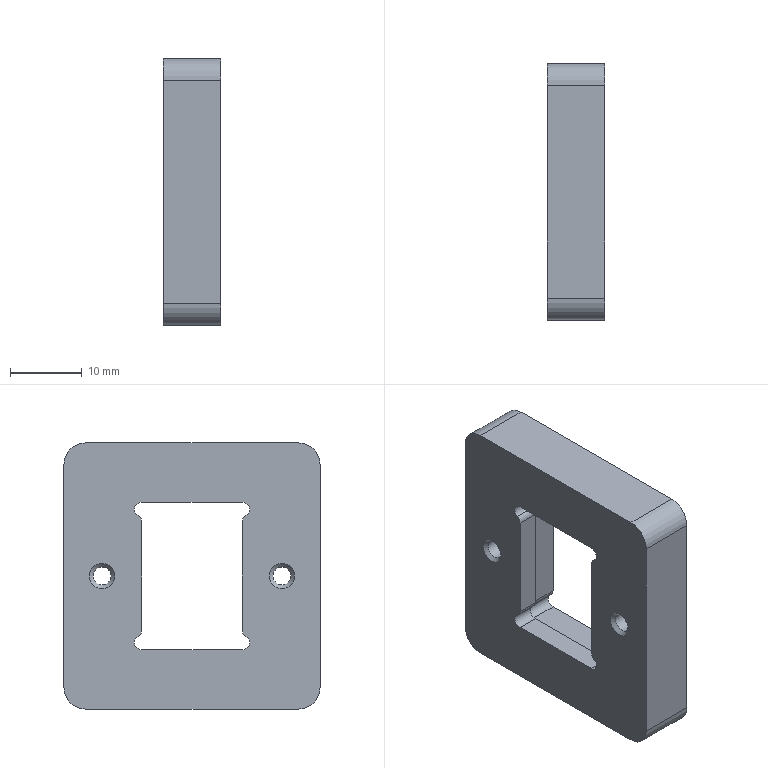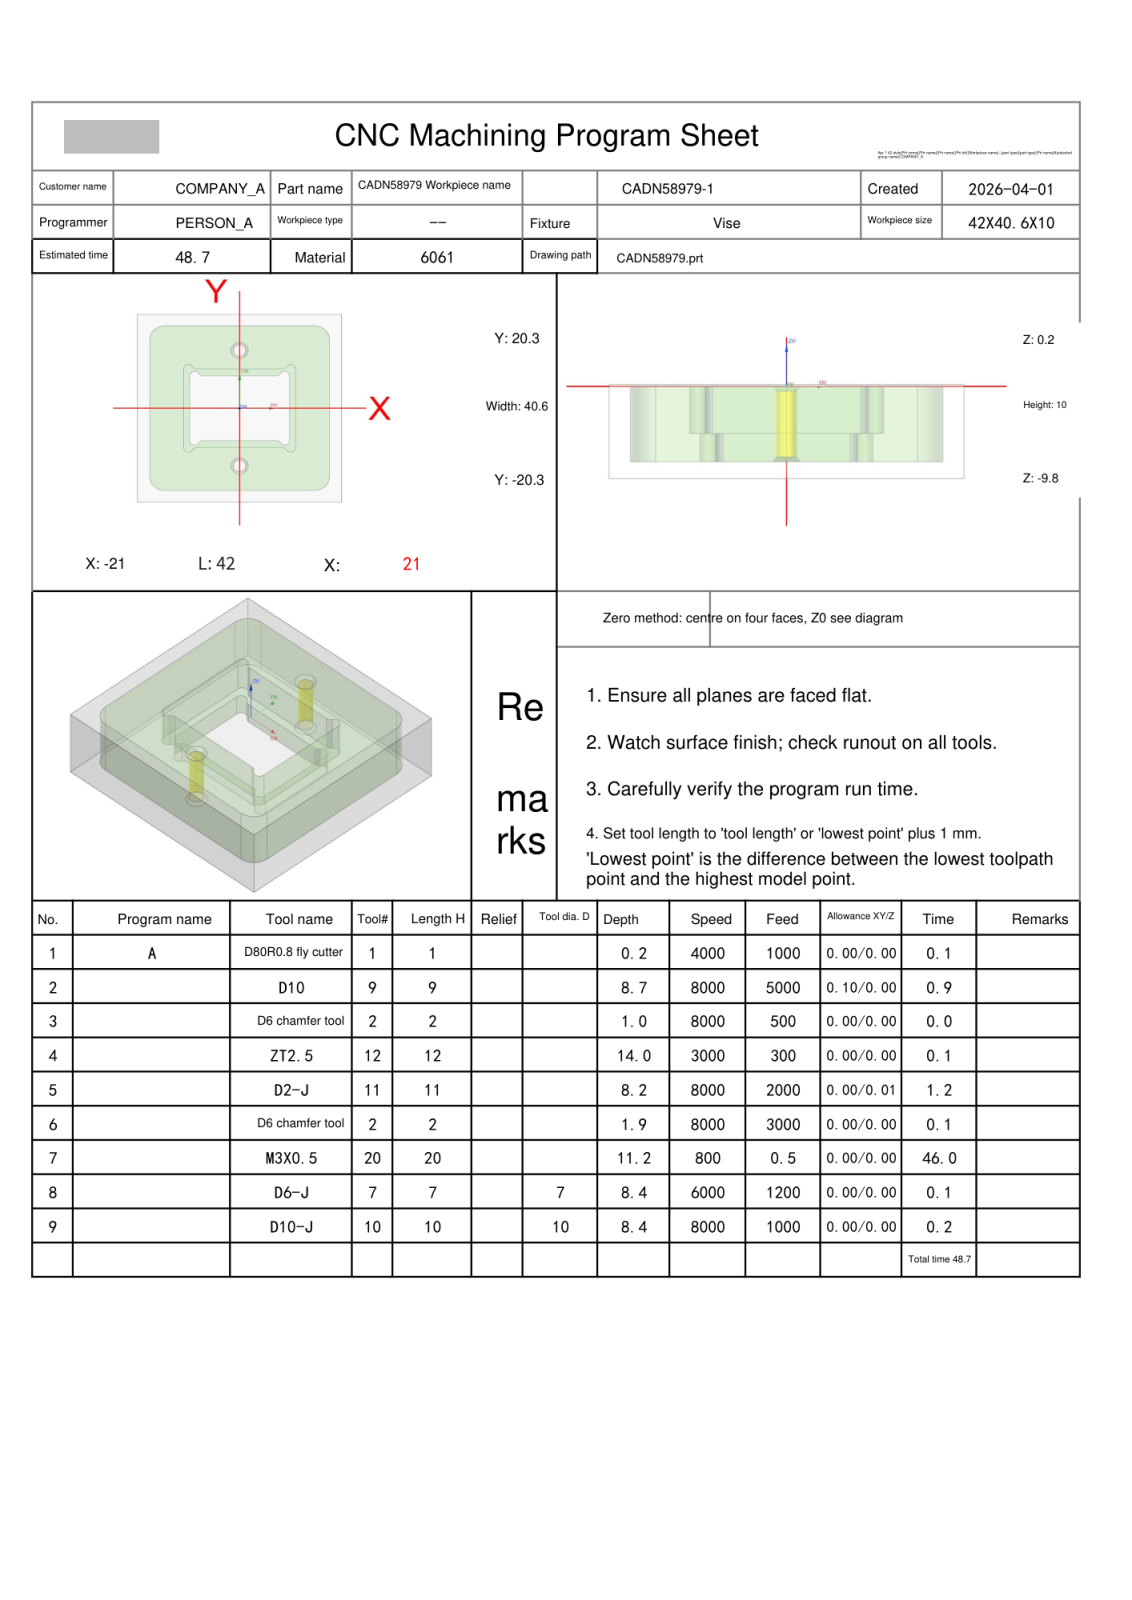NC program | NX | posted by the shop | part box 8 x 35.6 x 37 mm
Lines 3801 to 3954 of 3954:
N6 T02 M06
(D6 chamfer tool  D=6. R=0. H=02 ce=0.00 di=0.00)
G00 G90 G54 X.25 Y-19.928 M03 S8000
G43 H02 Z20.
M08
Z2.099
G01 Z-1.5 F3000.
G03 X.33 Y-19.628 I-.52 J.3
X.03 Y-19.108 I-.6 J0.0
G01 X0.0 Y-19.1
X-15.5
G02 X-19.8 Y-14.8 I0.0 J4.3
G01 Y14.8
G02 X-15.5 Y19.1 I4.3 J0.0
G01 X15.5
G02 X19.8 Y14.8 I0.0 J-4.3
G01 Y-14.8
G02 X15.5 Y-19.1 I-4.3 J0.0
G01 X0.0
X-.03 Y-19.108
G03 X-.33 Y-19.628 I.3 J-.52
X-.25 Y-19.928 I.6 J0.0
G01 Z2.099
G00 Z20.
X9.372 Y-.25
Z2.099
G01 Z-1.5
G03 X9.672 Y-.33 I.3 J.52
X10.192 Y-.03 I0.0 J.6
G01 X10.2 Y0.0
Y7.7
X9.879 Y7.486
X9.526 Y7.329
X9.153 Y7.232
X8.768 Y7.2
X-8.768
X-9.153 Y7.232
X-9.526 Y7.329
X-9.879 Y7.486
X-10.2 Y7.7
Y-7.7
X-9.879 Y-7.486
X-9.526 Y-7.329
X-9.153 Y-7.232
X-8.768 Y-7.2
X8.768
X9.153 Y-7.232
X9.526 Y-7.329
X9.879 Y-7.486
X10.2 Y-7.7
Y0.0
X10.192 Y.03
G03 X9.672 Y.33 I-.52 J-.3
X9.372 Y.25 I0.0 J-.6
G01 Z2.099
G00 Z20.
G00 G90 X0.0 Y-12.5 M03 S8000
Z20.
G98 G81 X0.0 Y-12.5 Z-1.75 R3. F500.
Y12.5
G80
G00 Z20.
G91 G28 Z0.0
M05
M09
G91 G28 Z0.0
M01
N7 T20 M06
(M3X0.5 D=2.5 DR_a=180 H=20)
G00 G90 G54 X0.0 Y-12.5 M03 S800
G43 H20 Z20.
M08
G95
G98 G84 X0.0 Y-12.5 Z-11. R.5 F.5 Q5.
Y12.5
G80
G94
G00 Z20.
G91 G28 Z0.0
M05
M09
G91 G28 Z0.0
M01
N8 T07 M06
(D6-J  D=6. R=0. H=07 ce=0.00 di=0.00)
G00 G90 G54 X-.2 Y-3.75 M03 S6000
G43 H07 Z20.
M08
Z-7.7
G01 Z-8.2 F600.
G41 D07
Y-3.8
G03 X0.0 Y-4. I.2 J0.0
G01 X7.25
Y4.
X-7.25
Y-4.
X0.0
X.5
G03 X.7 Y-3.8 I0.0 J.2
G01 G40 Y-3.75
Z-7.7
G00 Z20.
G00 G90 X-1. Y-4.4 M03 S6000
Z20.
Z-4.495
G01 Z-4.995 F1200.
G41 D07
Y-4.5
G03 X0.0 Y-5.5 I1. J0.0
G01 X8.5
Y5.5
X-8.5
Y-5.5
X0.0
X.5
G03 X1.5 Y-4.5 I0.0 J1.
G01 G40 Y-4.4
Z-4.495
G00 Z20.
G91 G28 Z0.0
M05
M09
G91 G28 Z0.0
M01
N9 T10 M06
(D10-J  D=10. R=0. H=10 ce=0.00 di=0.00)
G00 G90 G54 X16.51 Y-23.944 M03 S8000
G43 H10 Z20.
M08
Z-7.7
G01 Z-8.2 F1000.
G41 D10
X16.498 Y-23.744
G03 X15.5 Y-22.8 I-.998 J-.056
G01 X-15.5
G02 X-23.5 Y-14.8 I0.0 J8.
G01 Y14.8
G02 X-15.5 Y22.8 I8. J0.0
G01 X15.5
G02 X23.5 Y14.8 I0.0 J-8.
G01 Y-14.8
G02 X15.5 Y-22.8 I-8. J0.0
G01 X15.
G03 X14. Y-23.8 I0.0 J-1.
G01 G40 Y-24.
Z-7.7
G00 Z20.
M05
M09
G91 G28 Z0.0
G91 G28 Y0.0
M30
%